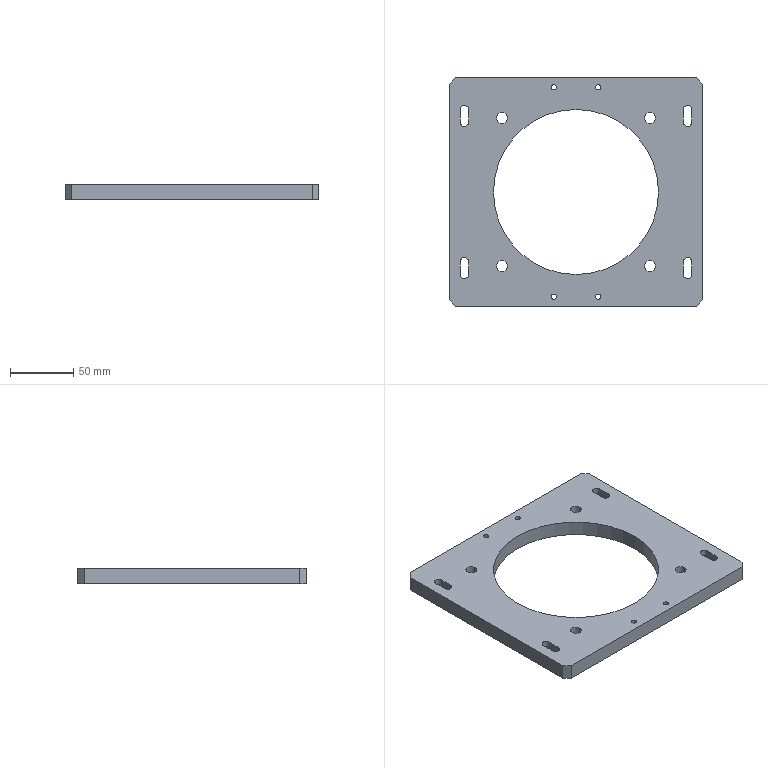Part | SolidWorks | features HoleWzd 4, MirrorPattern 2, Chamfer 1, Cut 1, Extrusion 1 | 1 solid | 64 faces | box 200 x 180 x 12 mm | volume 261071 mm3 | cylinder 34 | plane 30 | commonest cylinder face diameters 4.2 x8 6.6 x8 8.5 x8 11 x8 130 x2